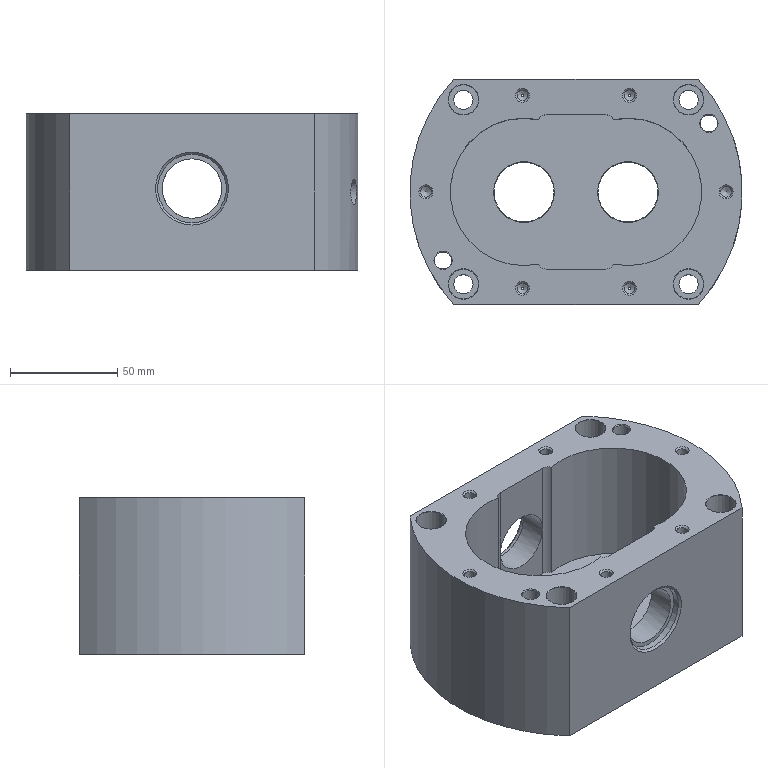NC program | NX | posted with a generic post | part box 155 x 105 x 73.2 mm
Lines 28870 to 29618 of 30727:
(FLOOR_WALL_1_COPY_COPY , TOOL : D12)
N57708 T12 M6
N57710 G54
N57712 G17 G0 G90 X-11.414 Y28.649 B0. C0. S4000 M3
N57714 G43 Z30. H12
N57716 Z-57.2
N57718 G94 G1 Z-60.2 F500.
N57720 G3 X-12.453 Y29.249 R1.2
N57722 G1 X12.453 F1000.
N57724 G3 X18.824 Y27.112 R6.75
N57726 G2 X38.981 Y23.399 R27.65
N57728 G1 X-38.981
N57730 G3 X-45.617 Y17.549 R27.65
N57732 G1 X45.617
N57734 G2 X49.303 Y11.699 R27.65
N57736 G1 X-49.303
N57738 G3 X-51.274 Y5.849 R27.65
N57740 G1 X51.274
N57742 G2 X51.9 Y0. R27.65
N57744 G1 X-51.9
N57746 G3 X-51.274 Y-5.85 R27.65
N57748 G1 X51.274
N57750 G2 X49.302 Y-11.7 R27.65
N57752 G1 X-49.302
N57754 G3 X-45.616 Y-17.55 R27.65
N57756 G1 X45.616
N57758 G2 X38.98 Y-23.4 R27.65
N57760 G1 X-38.98
N57762 G3 X-18.824 Y-27.112 R27.65
N57764 G2 X-12.452 Y-29.25 R6.75
N57766 G1 X12.452
N57768 G3 X12.693 Y-28.074 R1.2
N57770 G1 X12.332 Y-29.838
N57772 G3 X12.901 Y-29.648 R0.6 F500.
N57774 G2 X18.707 Y-27.701 R6.15 F1000.
N57776 G3 X18.707 Y27.701 R-28.25
N57778 G2 X12.729 Y29.85 R6.15
N57780 G1 X-12.729
N57782 G2 X-18.707 Y27.701 R6.15
N57784 G3 X-18.707 Y-27.701 R-28.25
N57786 G2 X-12.729 Y-29.85 R6.15
N57788 G1 X12.729
N57790 G2 X12.901 Y-29.648 R6.15
N57792 G3 X13.142 Y-28.473 R1.2
N57794 G1 X12.371 Y-26.154
N57796 Z-57.2
N57798 G0 Z30.
(ZLEVEL_PROFILE , TOOL : D12)
N57800 X-13.809 Y-22.52 S5000
N57802 Z-13.05
N57804 G1 Z-15.05 F1250.
N57806 X-14.839 Y-24.027
N57808 G3 X-14.93 Y-25.224 R1.2
N57810 G1 X-12.637 Y-30.
N57812 X12.637
N57814 X14.949 Y-25.184
N57816 G3 X14.858 Y-23.987 R1.2
N57818 G1 X13.835 Y-22.489
N57820 Z-13.05
N57822 G0 X-13.832 Y-22.491 Z-28.1
N57824 G1 Z-30.1
N57826 X-14.854 Y-24.026
N57828 G3 X-14.93 Y-25.224 R1.2
N57830 G1 X-14.907 Y-25.269
N57832 X-12.636 Y-30.
N57834 X12.636
N57836 X14.949 Y-25.183
N57838 G3 X14.858 Y-23.987 R1.2
N57840 G1 X13.834 Y-22.489
N57842 Z-28.1
N57844 G0 X-13.809 Y-22.52 Z-43.15
N57846 G1 Z-45.15
N57848 X-14.838 Y-24.027
N57850 G3 X-14.929 Y-25.223 R1.2
N57852 G1 X-12.636 Y-30.
N57854 X12.636
N57856 X14.946 Y-25.189
N57858 G3 X14.854 Y-23.992 R1.2
N57860 G1 X13.83 Y-22.493
N57862 Z-43.15
N57864 G0 X-13.808 Y-22.52 Z-58.2
N57866 G1 Z-60.2
N57868 X-14.838 Y-24.027
N57870 G3 X-14.929 Y-25.223 R1.2
N57872 G1 X-12.635 Y-30.
N57874 X12.635
N57876 X14.945 Y-25.189
N57878 G3 X14.854 Y-23.992 R1.2
N57880 G1 X13.829 Y-22.493
N57882 Z-58.2
N57884 G0 Z30.
N57886 X13.824 Y22.503
N57888 Z-13.05
N57890 G1 Z-15.05
N57892 X14.85 Y24.004
N57894 G3 X14.941 Y25.201 R1.2
N57896 G1 X12.636 Y30.001
N57898 X12.592 Y30.
N57900 X-12.592
N57902 X-12.636 Y30.001
N57904 X-14.93 Y25.224
N57906 G3 X-14.839 Y24.027 R1.2
N57908 G1 X-13.809 Y22.52
N57910 Z-13.05
N57912 G0 X13.823 Y22.503 Z-28.1
N57914 G1 Z-30.1
N57916 X14.85 Y24.004
N57918 G3 X14.941 Y25.201 R1.2
N57920 G1 X12.636 Y30.001
N57922 X12.592 Y30.
N57924 X-12.592
N57926 X-12.636 Y30.001
N57928 X-14.93 Y25.224
N57930 G3 X-14.839 Y24.027 R1.2
N57932 G1 X-13.809 Y22.52
N57934 Z-28.1
N57936 G0 X13.823 Y22.502 Z-43.15
N57938 G1 Z-45.15
N57940 X14.849 Y24.004
N57942 G3 X14.94 Y25.2 R1.2
N57944 G1 X12.636 Y30.
N57946 X-12.636
N57948 X-14.929 Y25.223
N57950 G3 X-14.838 Y24.027 R1.2
N57952 G1 X-13.809 Y22.52
N57954 Z-43.15
N57956 G0 X13.823 Y22.502 Z-58.2
N57958 G1 Z-60.2
N57960 X14.849 Y24.004
N57962 G3 X14.94 Y25.2 R1.2
N57964 G1 X12.635 Y30.
N57966 X-12.635
N57968 X-14.929 Y25.223
N57970 G3 X-14.838 Y24.027 R1.2
N57972 G1 X-13.808 Y22.52
N57974 Z-58.2
N57976 G0 Z30.
N57978 M5
(HOLE_MILLING_COPY_COPY_COPY_COPY , TOOL : D10)
N57980 T10 M6
N57982 G54
N57984 G17 G0 G90 X-52.5 Y43. B0. C0. S3000 M3
N57986 G43 Z30. H10
N57988 Z1.
N57990 G94 G3 X-51.55 Y42.05 R0.95 F2200.
N57992 X-50.6 Y43. R0.95
N57994 X-50.6 Y43. Z0.78 I-1.9 J0.
N57996 X-50.6 Y43. Z0.56 I-1.9 J0.
N57998 X-50.6 Y43. Z0.34 I-1.9 J0.
N58000 X-50.6 Y43. Z0.12 I-1.9 J0.
N58002 X-50.6 Y43. Z-0.1 I-1.9 J0.
N58004 X-50.6 Y43. Z-0.32 I-1.9 J0.
N58006 X-50.6 Y43. Z-0.54 I-1.9 J0.
N58008 X-50.6 Y43. Z-0.76 I-1.9 J0.
N58010 X-50.6 Y43. Z-0.98 I-1.9 J0.
N58012 X-50.6 Y43. Z-1.2 I-1.9 J0.
N58014 X-50.6 Y43. Z-1.42 I-1.9 J0.
N58016 X-50.6 Y43. Z-1.64 I-1.9 J0.
N58018 X-50.6 Y43. Z-1.86 I-1.9 J0.
N58020 X-50.6 Y43. Z-2.08 I-1.9 J0.
N58022 X-50.6 Y43. Z-2.3 I-1.9 J0.
N58024 X-50.6 Y43. Z-2.52 I-1.9 J0.
N58026 X-50.6 Y43. Z-2.74 I-1.9 J0.
N58028 X-50.6 Y43. Z-2.96 I-1.9 J0.
N58030 X-50.6 Y43. Z-3.18 I-1.9 J0.
N58032 X-50.6 Y43. Z-3.4 I-1.9 J0.
N58034 X-50.6 Y43. Z-3.62 I-1.9 J0.
N58036 X-50.6 Y43. Z-3.84 I-1.9 J0.
N58038 X-50.6 Y43. Z-4.06 I-1.9 J0.
N58040 X-50.6 Y43. Z-4.28 I-1.9 J0.
N58042 X-50.6 Y43. Z-4.5 I-1.9 J0.
N58044 X-50.6 Y43. Z-4.72 I-1.9 J0.
N58046 X-50.6 Y43. Z-4.94 I-1.9 J0.
N58048 X-50.6 Y43. Z-5.16 I-1.9 J0.
N58050 X-50.6 Y43. Z-5.38 I-1.9 J0.
N58052 X-50.6 Y43. Z-5.6 I-1.9 J0.
N58054 X-50.6 Y43. Z-5.82 I-1.9 J0.
N58056 X-50.6 Y43. Z-6.04 I-1.9 J0.
N58058 X-50.6 Y43. Z-6.26 I-1.9 J0.
N58060 X-50.6 Y43. Z-6.48 I-1.9 J0.
N58062 X-50.6 Y43. Z-6.7 I-1.9 J0.
N58064 X-50.6 Y43. Z-6.92 I-1.9 J0.
N58066 X-50.6 Y43. Z-7.14 I-1.9 J0.
N58068 X-50.6 Y43. Z-7.36 I-1.9 J0.
N58070 X-50.6 Y43. Z-7.58 I-1.9 J0.
N58072 X-50.6 Y43. Z-7.8 I-1.9 J0.
N58074 X-50.6 Y43. Z-8.02 I-1.9 J0.
N58076 X-50.6 Y43. Z-8.24 I-1.9 J0.
N58078 X-50.6 Y43. Z-8.46 I-1.9 J0.
N58080 X-50.6 Y43. Z-8.68 I-1.9 J0.
N58082 X-50.6 Y43. Z-8.9 I-1.9 J0.
N58084 X-50.6 Y43. Z-9.12 I-1.9 J0.
N58086 X-50.6 Y43. Z-9.34 I-1.9 J0.
N58088 X-50.6 Y43. Z-9.56 I-1.9 J0.
N58090 X-50.6 Y43. Z-9.78 I-1.9 J0.
N58092 X-50.6 Y43. Z-10. I-1.9 J0.
N58094 X-50.6 Y43. Z-10.22 I-1.9 J0.
N58096 X-50.6 Y43. Z-10.44 I-1.9 J0.
N58098 X-50.6 Y43. Z-10.66 I-1.9 J0.
N58100 X-50.6 Y43. Z-10.88 I-1.9 J0.
N58102 X-50.6 Y43. Z-11.1 I-1.9 J0.
N58104 X-50.6 Y43. Z-11.32 I-1.9 J0.
N58106 X-50.6 Y43. Z-11.54 I-1.9 J0.
N58108 X-50.6 Y43. Z-11.76 I-1.9 J0.
N58110 X-50.6 Y43. Z-11.98 I-1.9 J0.
N58112 X-50.6 Y43. Z-12.2 I-1.9 J0.
N58114 X-50.6 Y43. Z-12.42 I-1.9 J0.
N58116 X-50.6 Y43. Z-12.64 I-1.9 J0.
N58118 X-50.6 Y43. Z-12.86 I-1.9 J0.
N58120 X-50.6 Y43. Z-13.08 I-1.9 J0.
N58122 X-50.6 Y43. Z-13.3 I-1.9 J0.
N58124 X-50.6 Y43. Z-13.52 I-1.9 J0.
N58126 X-50.6 Y43. Z-13.74 I-1.9 J0.
N58128 X-50.6 Y43. Z-13.96 I-1.9 J0.
N58130 X-50.6 Y43. Z-14.18 I-1.9 J0.
N58132 X-50.6 Y43. Z-14.4 I-1.9 J0.
N58134 X-50.6 Y43. Z-14.62 I-1.9 J0.
N58136 X-50.6 Y43. Z-14.84 I-1.9 J0.
N58138 X-50.6 Y43. Z-15.06 I-1.9 J0.
N58140 X-50.6 Y43. Z-15.28 I-1.9 J0.
N58142 X-50.6 Y43. Z-15.5 I-1.9 J0.
N58144 X-50.6 Y43. Z-15.72 I-1.9 J0.
N58146 X-50.6 Y43. Z-15.94 I-1.9 J0.
N58148 X-50.6 Y43. Z-16.16 I-1.9 J0.
N58150 X-50.6 Y43. Z-16.38 I-1.9 J0.
N58152 X-50.6 Y43. Z-16.6 I-1.9 J0.
N58154 X-50.6 Y43. Z-16.82 I-1.9 J0.
N58156 X-50.6 Y43. Z-17.04 I-1.9 J0.
N58158 X-50.6 Y43. Z-17.26 I-1.9 J0.
N58160 X-50.6 Y43. Z-17.48 I-1.9 J0.
N58162 X-50.6 Y43. Z-17.7 I-1.9 J0.
N58164 X-50.6 Y43. Z-17.92 I-1.9 J0.
N58166 X-50.6 Y43. Z-18.14 I-1.9 J0.
N58168 X-50.6 Y43. Z-18.36 I-1.9 J0.
N58170 X-50.6 Y43. Z-18.58 I-1.9 J0.
N58172 X-50.6 Y43. Z-18.8 I-1.9 J0.
N58174 X-50.6 Y43. Z-19.02 I-1.9 J0.
N58176 X-50.6 Y43. Z-19.24 I-1.9 J0.
N58178 X-50.6 Y43. Z-19.46 I-1.9 J0.
N58180 X-50.6 Y43. Z-19.68 I-1.9 J0.
N58182 X-50.6 Y43. Z-19.9 I-1.9 J0.
N58184 X-50.6 Y43. Z-20.12 I-1.9 J0.
N58186 X-50.6 Y43. Z-20.34 I-1.9 J0.
N58188 X-50.6 Y43. Z-20.56 I-1.9 J0.
N58190 X-50.6 Y43. Z-20.78 I-1.9 J0.
N58192 X-50.6 Y43. Z-21. I-1.9 J0.
N58194 X-50.6 Y43. Z-21.22 I-1.9 J0.
N58196 X-50.6 Y43. Z-21.44 I-1.9 J0.
N58198 X-50.6 Y43. Z-21.66 I-1.9 J0.
N58200 X-50.6 Y43. Z-21.88 I-1.9 J0.
N58202 X-50.6 Y43. Z-22.1 I-1.9 J0.
N58204 X-50.6 Y43. Z-22.32 I-1.9 J0.
N58206 X-50.6 Y43. Z-22.54 I-1.9 J0.
N58208 X-50.6 Y43. Z-22.76 I-1.9 J0.
N58210 X-50.6 Y43. Z-22.98 I-1.9 J0.
N58212 X-50.6 Y43. Z-23.2 I-1.9 J0.
N58214 X-50.6 Y43. Z-23.42 I-1.9 J0.
N58216 X-50.6 Y43. Z-23.64 I-1.9 J0.
N58218 X-50.6 Y43. Z-23.86 I-1.9 J0.
N58220 X-50.6 Y43. Z-24.08 I-1.9 J0.
N58222 X-50.6 Y43. Z-24.3 I-1.9 J0.
N58224 X-50.6 Y43. Z-24.52 I-1.9 J0.
N58226 X-50.6 Y43. Z-24.74 I-1.9 J0.
N58228 X-50.6 Y43. Z-24.96 I-1.9 J0.
N58230 X-50.6 Y43. Z-25.18 I-1.9 J0.
N58232 X-50.6 Y43. Z-25.4 I-1.9 J0.
N58234 X-50.6 Y43. Z-25.62 I-1.9 J0.
N58236 X-50.6 Y43. Z-25.84 I-1.9 J0.
N58238 X-50.6 Y43. Z-26.06 I-1.9 J0.
N58240 X-50.6 Y43. Z-26.28 I-1.9 J0.
N58242 X-50.6 Y43. Z-26.5 I-1.9 J0.
N58244 X-50.6 Y43. Z-26.72 I-1.9 J0.
N58246 X-50.6 Y43. Z-26.94 I-1.9 J0.
N58248 X-50.6 Y43. Z-27.16 I-1.9 J0.
N58250 X-50.6 Y43. Z-27.38 I-1.9 J0.
N58252 X-50.6 Y43. Z-27.6 I-1.9 J0.
N58254 X-50.6 Y43. Z-27.82 I-1.9 J0.
N58256 X-50.6 Y43. Z-28.04 I-1.9 J0.
N58258 X-50.6 Y43. Z-28.26 I-1.9 J0.
N58260 X-50.6 Y43. Z-28.48 I-1.9 J0.
N58262 X-50.6 Y43. Z-28.7 I-1.9 J0.
N58264 X-50.6 Y43. Z-28.92 I-1.9 J0.
N58266 X-50.6 Y43. Z-29.14 I-1.9 J0.
N58268 X-50.6 Y43. Z-29.36 I-1.9 J0.
N58270 X-50.6 Y43. Z-29.58 I-1.9 J0.
N58272 X-50.6 Y43. Z-29.8 I-1.9 J0.
N58274 X-50.902 Y41.973 Z-30. R-1.9
N58276 X-51.473 Y44.598 R1.9
N58278 X-50.902 Y41.973 R-1.9
N58280 X-51.187 Y43.286 R0.95
N58282 X-52.5 Y43. R0.95
N58284 G0 Z30.
N58286 Y-43.
N58288 Z1.
N58290 G3 X-51.55 Y-43.95 R0.95
N58292 X-50.6 Y-43. R0.95
N58294 X-50.6 Y-43. Z0.78 I-1.9 J0.
N58296 X-50.6 Y-43. Z0.56 I-1.9 J0.
N58298 X-50.6 Y-43. Z0.34 I-1.9 J0.
N58300 X-50.6 Y-43. Z0.12 I-1.9 J0.
N58302 X-50.6 Y-43. Z-0.1 I-1.9 J0.
N58304 X-50.6 Y-43. Z-0.32 I-1.9 J0.
N58306 X-50.6 Y-43. Z-0.54 I-1.9 J0.
N58308 X-50.6 Y-43. Z-0.76 I-1.9 J0.
N58310 X-50.6 Y-43. Z-0.98 I-1.9 J0.
N58312 X-50.6 Y-43. Z-1.2 I-1.9 J0.
N58314 X-50.6 Y-43. Z-1.42 I-1.9 J0.
N58316 X-50.6 Y-43. Z-1.64 I-1.9 J0.
N58318 X-50.6 Y-43. Z-1.86 I-1.9 J0.
N58320 X-50.6 Y-43. Z-2.08 I-1.9 J0.
N58322 X-50.6 Y-43. Z-2.3 I-1.9 J0.
N58324 X-50.6 Y-43. Z-2.52 I-1.9 J0.
N58326 X-50.6 Y-43. Z-2.74 I-1.9 J0.
N58328 X-50.6 Y-43. Z-2.96 I-1.9 J0.
N58330 X-50.6 Y-43. Z-3.18 I-1.9 J0.
N58332 X-50.6 Y-43. Z-3.4 I-1.9 J0.
N58334 X-50.6 Y-43. Z-3.62 I-1.9 J0.
N58336 X-50.6 Y-43. Z-3.84 I-1.9 J0.
N58338 X-50.6 Y-43. Z-4.06 I-1.9 J0.
N58340 X-50.6 Y-43. Z-4.28 I-1.9 J0.
N58342 X-50.6 Y-43. Z-4.5 I-1.9 J0.
N58344 X-50.6 Y-43. Z-4.72 I-1.9 J0.
N58346 X-50.6 Y-43. Z-4.94 I-1.9 J0.
N58348 X-50.6 Y-43. Z-5.16 I-1.9 J0.
N58350 X-50.6 Y-43. Z-5.38 I-1.9 J0.
N58352 X-50.6 Y-43. Z-5.6 I-1.9 J0.
N58354 X-50.6 Y-43. Z-5.82 I-1.9 J0.
N58356 X-50.6 Y-43. Z-6.04 I-1.9 J0.
N58358 X-50.6 Y-43. Z-6.26 I-1.9 J0.
N58360 X-50.6 Y-43. Z-6.48 I-1.9 J0.
N58362 X-50.6 Y-43. Z-6.7 I-1.9 J0.
N58364 X-50.6 Y-43. Z-6.92 I-1.9 J0.
N58366 X-50.6 Y-43. Z-7.14 I-1.9 J0.
N58368 X-50.6 Y-43. Z-7.36 I-1.9 J0.
N58370 X-50.6 Y-43. Z-7.58 I-1.9 J0.
N58372 X-50.6 Y-43. Z-7.8 I-1.9 J0.
N58374 X-50.6 Y-43. Z-8.02 I-1.9 J0.
N58376 X-50.6 Y-43. Z-8.24 I-1.9 J0.
N58378 X-50.6 Y-43. Z-8.46 I-1.9 J0.
N58380 X-50.6 Y-43. Z-8.68 I-1.9 J0.
N58382 X-50.6 Y-43. Z-8.9 I-1.9 J0.
N58384 X-50.6 Y-43. Z-9.12 I-1.9 J0.
N58386 X-50.6 Y-43. Z-9.34 I-1.9 J0.
N58388 X-50.6 Y-43. Z-9.56 I-1.9 J0.
N58390 X-50.6 Y-43. Z-9.78 I-1.9 J0.
N58392 X-50.6 Y-43. Z-10. I-1.9 J0.
N58394 X-50.6 Y-43. Z-10.22 I-1.9 J0.
N58396 X-50.6 Y-43. Z-10.44 I-1.9 J0.
N58398 X-50.6 Y-43. Z-10.66 I-1.9 J0.
N58400 X-50.6 Y-43. Z-10.88 I-1.9 J0.
N58402 X-50.6 Y-43. Z-11.1 I-1.9 J0.
N58404 X-50.6 Y-43. Z-11.32 I-1.9 J0.
N58406 X-50.6 Y-43. Z-11.54 I-1.9 J0.
N58408 X-50.6 Y-43. Z-11.76 I-1.9 J0.
N58410 X-50.6 Y-43. Z-11.98 I-1.9 J0.
N58412 X-50.6 Y-43. Z-12.2 I-1.9 J0.
N58414 X-50.6 Y-43. Z-12.42 I-1.9 J0.
N58416 X-50.6 Y-43. Z-12.64 I-1.9 J0.
N58418 X-50.6 Y-43. Z-12.86 I-1.9 J0.
N58420 X-50.6 Y-43. Z-13.08 I-1.9 J0.
N58422 X-50.6 Y-43. Z-13.3 I-1.9 J0.
N58424 X-50.6 Y-43. Z-13.52 I-1.9 J0.
N58426 X-50.6 Y-43. Z-13.74 I-1.9 J0.
N58428 X-50.6 Y-43. Z-13.96 I-1.9 J0.
N58430 X-50.6 Y-43. Z-14.18 I-1.9 J0.
N58432 X-50.6 Y-43. Z-14.4 I-1.9 J0.
N58434 X-50.6 Y-43. Z-14.62 I-1.9 J0.
N58436 X-50.6 Y-43. Z-14.84 I-1.9 J0.
N58438 X-50.6 Y-43. Z-15.06 I-1.9 J0.
N58440 X-50.6 Y-43. Z-15.28 I-1.9 J0.
N58442 X-50.6 Y-43. Z-15.5 I-1.9 J0.
N58444 X-50.6 Y-43. Z-15.72 I-1.9 J0.
N58446 X-50.6 Y-43. Z-15.94 I-1.9 J0.
N58448 X-50.6 Y-43. Z-16.16 I-1.9 J0.
N58450 X-50.6 Y-43. Z-16.38 I-1.9 J0.
N58452 X-50.6 Y-43. Z-16.6 I-1.9 J0.
N58454 X-50.6 Y-43. Z-16.82 I-1.9 J0.
N58456 X-50.6 Y-43. Z-17.04 I-1.9 J0.
N58458 X-50.6 Y-43. Z-17.26 I-1.9 J0.
N58460 X-50.6 Y-43. Z-17.48 I-1.9 J0.
N58462 X-50.6 Y-43. Z-17.7 I-1.9 J0.
N58464 X-50.6 Y-43. Z-17.92 I-1.9 J0.
N58466 X-50.6 Y-43. Z-18.14 I-1.9 J0.
N58468 X-50.6 Y-43. Z-18.36 I-1.9 J0.
N58470 X-50.6 Y-43. Z-18.58 I-1.9 J0.
N58472 X-50.6 Y-43. Z-18.8 I-1.9 J0.
N58474 X-50.6 Y-43. Z-19.02 I-1.9 J0.
N58476 X-50.6 Y-43. Z-19.24 I-1.9 J0.
N58478 X-50.6 Y-43. Z-19.46 I-1.9 J0.
N58480 X-50.6 Y-43. Z-19.68 I-1.9 J0.
N58482 X-50.6 Y-43. Z-19.9 I-1.9 J0.
N58484 X-50.6 Y-43. Z-20.12 I-1.9 J0.
N58486 X-50.6 Y-43. Z-20.34 I-1.9 J0.
N58488 X-50.6 Y-43. Z-20.56 I-1.9 J0.
N58490 X-50.6 Y-43. Z-20.78 I-1.9 J0.
N58492 X-50.6 Y-43. Z-21. I-1.9 J0.
N58494 X-50.6 Y-43. Z-21.22 I-1.9 J0.
N58496 X-50.6 Y-43. Z-21.44 I-1.9 J0.
N58498 X-50.6 Y-43. Z-21.66 I-1.9 J0.
N58500 X-50.6 Y-43. Z-21.88 I-1.9 J0.
N58502 X-50.6 Y-43. Z-22.1 I-1.9 J0.
N58504 X-50.6 Y-43. Z-22.32 I-1.9 J0.
N58506 X-50.6 Y-43. Z-22.54 I-1.9 J0.
N58508 X-50.6 Y-43. Z-22.76 I-1.9 J0.
N58510 X-50.6 Y-43. Z-22.98 I-1.9 J0.
N58512 X-50.6 Y-43. Z-23.2 I-1.9 J0.
N58514 X-50.6 Y-43. Z-23.42 I-1.9 J0.
N58516 X-50.6 Y-43. Z-23.64 I-1.9 J0.
N58518 X-50.6 Y-43. Z-23.86 I-1.9 J0.
N58520 X-50.6 Y-43. Z-24.08 I-1.9 J0.
N58522 X-50.6 Y-43. Z-24.3 I-1.9 J0.
N58524 X-50.6 Y-43. Z-24.52 I-1.9 J0.
N58526 X-50.6 Y-43. Z-24.74 I-1.9 J0.
N58528 X-50.6 Y-43. Z-24.96 I-1.9 J0.
N58530 X-50.6 Y-43. Z-25.18 I-1.9 J0.
N58532 X-50.6 Y-43. Z-25.4 I-1.9 J0.
N58534 X-50.6 Y-43. Z-25.62 I-1.9 J0.
N58536 X-50.6 Y-43. Z-25.84 I-1.9 J0.
N58538 X-50.6 Y-43. Z-26.06 I-1.9 J0.
N58540 X-50.6 Y-43. Z-26.28 I-1.9 J0.
N58542 X-50.6 Y-43. Z-26.5 I-1.9 J0.
N58544 X-50.6 Y-43. Z-26.72 I-1.9 J0.
N58546 X-50.6 Y-43. Z-26.94 I-1.9 J0.
N58548 X-50.6 Y-43. Z-27.16 I-1.9 J0.
N58550 X-50.6 Y-43. Z-27.38 I-1.9 J0.
N58552 X-50.6 Y-43. Z-27.6 I-1.9 J0.
N58554 X-50.6 Y-43. Z-27.82 I-1.9 J0.
N58556 X-50.6 Y-43. Z-28.04 I-1.9 J0.
N58558 X-50.6 Y-43. Z-28.26 I-1.9 J0.
N58560 X-50.6 Y-43. Z-28.48 I-1.9 J0.
N58562 X-50.6 Y-43. Z-28.7 I-1.9 J0.
N58564 X-50.6 Y-43. Z-28.92 I-1.9 J0.
N58566 X-50.6 Y-43. Z-29.14 I-1.9 J0.
N58568 X-50.6 Y-43. Z-29.36 I-1.9 J0.
N58570 X-50.6 Y-43. Z-29.58 I-1.9 J0.
N58572 X-50.6 Y-43. Z-29.8 I-1.9 J0.
N58574 X-50.902 Y-44.027 Z-30. R-1.9
N58576 X-51.473 Y-41.402 R1.9
N58578 X-50.902 Y-44.027 R-1.9
N58580 X-51.187 Y-42.714 R0.95
N58582 X-52.5 Y-43. R0.95
N58584 G0 Z30.
N58586 X52.5
N58588 Z1.
N58590 G3 X53.45 Y-43.95 R0.95
N58592 X54.4 Y-43. R0.95
N58594 X54.4 Y-43. Z0.78 I-1.9 J0.
N58596 X54.4 Y-43. Z0.56 I-1.9 J0.
N58598 X54.4 Y-43. Z0.34 I-1.9 J0.
N58600 X54.4 Y-43. Z0.12 I-1.9 J0.
N58602 X54.4 Y-43. Z-0.1 I-1.9 J0.
N58604 X54.4 Y-43. Z-0.32 I-1.9 J0.
N58606 X54.4 Y-43. Z-0.54 I-1.9 J0.
N58608 X54.4 Y-43. Z-0.76 I-1.9 J0.
N58610 X54.4 Y-43. Z-0.98 I-1.9 J0.
N58612 X54.4 Y-43. Z-1.2 I-1.9 J0.
N58614 X54.4 Y-43. Z-1.42 I-1.9 J0.
N58616 X54.4 Y-43. Z-1.64 I-1.9 J0.
N58618 X54.4 Y-43. Z-1.86 I-1.9 J0.
N58620 X54.4 Y-43. Z-2.08 I-1.9 J0.
N58622 X54.4 Y-43. Z-2.3 I-1.9 J0.
N58624 X54.4 Y-43. Z-2.52 I-1.9 J0.
N58626 X54.4 Y-43. Z-2.74 I-1.9 J0.
N58628 X54.4 Y-43. Z-2.96 I-1.9 J0.
N58630 X54.4 Y-43. Z-3.18 I-1.9 J0.
N58632 X54.4 Y-43. Z-3.4 I-1.9 J0.
N58634 X54.4 Y-43. Z-3.62 I-1.9 J0.
N58636 X54.4 Y-43. Z-3.84 I-1.9 J0.
N58638 X54.4 Y-43. Z-4.06 I-1.9 J0.
N58640 X54.4 Y-43. Z-4.28 I-1.9 J0.
N58642 X54.4 Y-43. Z-4.5 I-1.9 J0.
N58644 X54.4 Y-43. Z-4.72 I-1.9 J0.
N58646 X54.4 Y-43. Z-4.94 I-1.9 J0.
N58648 X54.4 Y-43. Z-5.16 I-1.9 J0.
N58650 X54.4 Y-43. Z-5.38 I-1.9 J0.
N58652 X54.4 Y-43. Z-5.6 I-1.9 J0.
N58654 X54.4 Y-43. Z-5.82 I-1.9 J0.
N58656 X54.4 Y-43. Z-6.04 I-1.9 J0.
N58658 X54.4 Y-43. Z-6.26 I-1.9 J0.
N58660 X54.4 Y-43. Z-6.48 I-1.9 J0.
N58662 X54.4 Y-43. Z-6.7 I-1.9 J0.
N58664 X54.4 Y-43. Z-6.92 I-1.9 J0.
N58666 X54.4 Y-43. Z-7.14 I-1.9 J0.
N58668 X54.4 Y-43. Z-7.36 I-1.9 J0.
N58670 X54.4 Y-43. Z-7.58 I-1.9 J0.
N58672 X54.4 Y-43. Z-7.8 I-1.9 J0.
N58674 X54.4 Y-43. Z-8.02 I-1.9 J0.
N58676 X54.4 Y-43. Z-8.24 I-1.9 J0.
N58678 X54.4 Y-43. Z-8.46 I-1.9 J0.
N58680 X54.4 Y-43. Z-8.68 I-1.9 J0.
N58682 X54.4 Y-43. Z-8.9 I-1.9 J0.
N58684 X54.4 Y-43. Z-9.12 I-1.9 J0.
N58686 X54.4 Y-43. Z-9.34 I-1.9 J0.
N58688 X54.4 Y-43. Z-9.56 I-1.9 J0.
N58690 X54.4 Y-43. Z-9.78 I-1.9 J0.
N58692 X54.4 Y-43. Z-10. I-1.9 J0.
N58694 X54.4 Y-43. Z-10.22 I-1.9 J0.
N58696 X54.4 Y-43. Z-10.44 I-1.9 J0.
N58698 X54.4 Y-43. Z-10.66 I-1.9 J0.
N58700 X54.4 Y-43. Z-10.88 I-1.9 J0.
N58702 X54.4 Y-43. Z-11.1 I-1.9 J0.
N58704 X54.4 Y-43. Z-11.32 I-1.9 J0.
N58706 X54.4 Y-43. Z-11.54 I-1.9 J0.
N58708 X54.4 Y-43. Z-11.76 I-1.9 J0.
N58710 X54.4 Y-43. Z-11.98 I-1.9 J0.
N58712 X54.4 Y-43. Z-12.2 I-1.9 J0.
N58714 X54.4 Y-43. Z-12.42 I-1.9 J0.
N58716 X54.4 Y-43. Z-12.64 I-1.9 J0.
N58718 X54.4 Y-43. Z-12.86 I-1.9 J0.
N58720 X54.4 Y-43. Z-13.08 I-1.9 J0.
N58722 X54.4 Y-43. Z-13.3 I-1.9 J0.
N58724 X54.4 Y-43. Z-13.52 I-1.9 J0.
N58726 X54.4 Y-43. Z-13.74 I-1.9 J0.
N58728 X54.4 Y-43. Z-13.96 I-1.9 J0.
N58730 X54.4 Y-43. Z-14.18 I-1.9 J0.
N58732 X54.4 Y-43. Z-14.4 I-1.9 J0.
N58734 X54.4 Y-43. Z-14.62 I-1.9 J0.
N58736 X54.4 Y-43. Z-14.84 I-1.9 J0.
N58738 X54.4 Y-43. Z-15.06 I-1.9 J0.
N58740 X54.4 Y-43. Z-15.28 I-1.9 J0.
N58742 X54.4 Y-43. Z-15.5 I-1.9 J0.
N58744 X54.4 Y-43. Z-15.72 I-1.9 J0.
N58746 X54.4 Y-43. Z-15.94 I-1.9 J0.
N58748 X54.4 Y-43. Z-16.16 I-1.9 J0.
N58750 X54.4 Y-43. Z-16.38 I-1.9 J0.
N58752 X54.4 Y-43. Z-16.6 I-1.9 J0.
N58754 X54.4 Y-43. Z-16.82 I-1.9 J0.
N58756 X54.4 Y-43. Z-17.04 I-1.9 J0.
N58758 X54.4 Y-43. Z-17.26 I-1.9 J0.
N58760 X54.4 Y-43. Z-17.48 I-1.9 J0.
N58762 X54.4 Y-43. Z-17.7 I-1.9 J0.
N58764 X54.4 Y-43. Z-17.92 I-1.9 J0.
N58766 X54.4 Y-43. Z-18.14 I-1.9 J0.
N58768 X54.4 Y-43. Z-18.36 I-1.9 J0.
N58770 X54.4 Y-43. Z-18.58 I-1.9 J0.
N58772 X54.4 Y-43. Z-18.8 I-1.9 J0.
N58774 X54.4 Y-43. Z-19.02 I-1.9 J0.
N58776 X54.4 Y-43. Z-19.24 I-1.9 J0.
N58778 X54.4 Y-43. Z-19.46 I-1.9 J0.
N58780 X54.4 Y-43. Z-19.68 I-1.9 J0.
N58782 X54.4 Y-43. Z-19.9 I-1.9 J0.
N58784 X54.4 Y-43. Z-20.12 I-1.9 J0.
N58786 X54.4 Y-43. Z-20.34 I-1.9 J0.
N58788 X54.4 Y-43. Z-20.56 I-1.9 J0.
N58790 X54.4 Y-43. Z-20.78 I-1.9 J0.
N58792 X54.4 Y-43. Z-21. I-1.9 J0.
N58794 X54.4 Y-43. Z-21.22 I-1.9 J0.
N58796 X54.4 Y-43. Z-21.44 I-1.9 J0.
N58798 X54.4 Y-43. Z-21.66 I-1.9 J0.
N58800 X54.4 Y-43. Z-21.88 I-1.9 J0.
N58802 X54.4 Y-43. Z-22.1 I-1.9 J0.
N58804 X54.4 Y-43. Z-22.32 I-1.9 J0.
N58806 X54.4 Y-43. Z-22.54 I-1.9 J0.
N58808 X54.4 Y-43. Z-22.76 I-1.9 J0.
N58810 X54.4 Y-43. Z-22.98 I-1.9 J0.
N58812 X54.4 Y-43. Z-23.2 I-1.9 J0.
N58814 X54.4 Y-43. Z-23.42 I-1.9 J0.
N58816 X54.4 Y-43. Z-23.64 I-1.9 J0.
N58818 X54.4 Y-43. Z-23.86 I-1.9 J0.
N58820 X54.4 Y-43. Z-24.08 I-1.9 J0.
N58822 X54.4 Y-43. Z-24.3 I-1.9 J0.
N58824 X54.4 Y-43. Z-24.52 I-1.9 J0.
N58826 X54.4 Y-43. Z-24.74 I-1.9 J0.
N58828 X54.4 Y-43. Z-24.96 I-1.9 J0.
N58830 X54.4 Y-43. Z-25.18 I-1.9 J0.
N58832 X54.4 Y-43. Z-25.4 I-1.9 J0.
N58834 X54.4 Y-43. Z-25.62 I-1.9 J0.
N58836 X54.4 Y-43. Z-25.84 I-1.9 J0.
N58838 X54.4 Y-43. Z-26.06 I-1.9 J0.
N58840 X54.4 Y-43. Z-26.28 I-1.9 J0.
N58842 X54.4 Y-43. Z-26.5 I-1.9 J0.
N58844 X54.4 Y-43. Z-26.72 I-1.9 J0.
N58846 X54.4 Y-43. Z-26.94 I-1.9 J0.
N58848 X54.4 Y-43. Z-27.16 I-1.9 J0.
N58850 X54.4 Y-43. Z-27.38 I-1.9 J0.
N58852 X54.4 Y-43. Z-27.6 I-1.9 J0.
N58854 X54.4 Y-43. Z-27.82 I-1.9 J0.
N58856 X54.4 Y-43. Z-28.04 I-1.9 J0.
N58858 X54.4 Y-43. Z-28.26 I-1.9 J0.
N58860 X54.4 Y-43. Z-28.48 I-1.9 J0.
N58862 X54.4 Y-43. Z-28.7 I-1.9 J0.
N58864 X54.4 Y-43. Z-28.92 I-1.9 J0.
N58866 X54.4 Y-43. Z-29.14 I-1.9 J0.
N58868 X54.4 Y-43. Z-29.36 I-1.9 J0.
N58870 X54.4 Y-43. Z-29.58 I-1.9 J0.
N58872 X54.4 Y-43. Z-29.8 I-1.9 J0.
N58874 X54.098 Y-44.027 Z-30. R-1.9
N58876 X53.527 Y-41.402 R1.9
N58878 X54.098 Y-44.027 R-1.9
N58880 X53.813 Y-42.714 R0.95
N58882 X52.5 Y-43. R0.95
N58884 G0 Z30.
N58886 Y43.
N58888 Z1.
N58890 G3 X53.45 Y42.05 R0.95
N58892 X54.4 Y43. R0.95
N58894 X54.4 Y43. Z0.78 I-1.9 J0.
N58896 X54.4 Y43. Z0.56 I-1.9 J0.
N58898 X54.4 Y43. Z0.34 I-1.9 J0.
N58900 X54.4 Y43. Z0.12 I-1.9 J0.
N58902 X54.4 Y43. Z-0.1 I-1.9 J0.
N58904 X54.4 Y43. Z-0.32 I-1.9 J0.
N58906 X54.4 Y43. Z-0.54 I-1.9 J0.
N58908 X54.4 Y43. Z-0.76 I-1.9 J0.
N58910 X54.4 Y43. Z-0.98 I-1.9 J0.
N58912 X54.4 Y43. Z-1.2 I-1.9 J0.
N58914 X54.4 Y43. Z-1.42 I-1.9 J0.
N58916 X54.4 Y43. Z-1.64 I-1.9 J0.
N58918 X54.4 Y43. Z-1.86 I-1.9 J0.
N58920 X54.4 Y43. Z-2.08 I-1.9 J0.
N58922 X54.4 Y43. Z-2.3 I-1.9 J0.
N58924 X54.4 Y43. Z-2.52 I-1.9 J0.
N58926 X54.4 Y43. Z-2.74 I-1.9 J0.
N58928 X54.4 Y43. Z-2.96 I-1.9 J0.
N58930 X54.4 Y43. Z-3.18 I-1.9 J0.
N58932 X54.4 Y43. Z-3.4 I-1.9 J0.
N58934 X54.4 Y43. Z-3.62 I-1.9 J0.
N58936 X54.4 Y43. Z-3.84 I-1.9 J0.
N58938 X54.4 Y43. Z-4.06 I-1.9 J0.
N58940 X54.4 Y43. Z-4.28 I-1.9 J0.
N58942 X54.4 Y43. Z-4.5 I-1.9 J0.
N58944 X54.4 Y43. Z-4.72 I-1.9 J0.
N58946 X54.4 Y43. Z-4.94 I-1.9 J0.
N58948 X54.4 Y43. Z-5.16 I-1.9 J0.
N58950 X54.4 Y43. Z-5.38 I-1.9 J0.
N58952 X54.4 Y43. Z-5.6 I-1.9 J0.
N58954 X54.4 Y43. Z-5.82 I-1.9 J0.
N58956 X54.4 Y43. Z-6.04 I-1.9 J0.
N58958 X54.4 Y43. Z-6.26 I-1.9 J0.
N58960 X54.4 Y43. Z-6.48 I-1.9 J0.
N58962 X54.4 Y43. Z-6.7 I-1.9 J0.
N58964 X54.4 Y43. Z-6.92 I-1.9 J0.
N58966 X54.4 Y43. Z-7.14 I-1.9 J0.
N58968 X54.4 Y43. Z-7.36 I-1.9 J0.
N58970 X54.4 Y43. Z-7.58 I-1.9 J0.
N58972 X54.4 Y43. Z-7.8 I-1.9 J0.
N58974 X54.4 Y43. Z-8.02 I-1.9 J0.
N58976 X54.4 Y43. Z-8.24 I-1.9 J0.
N58978 X54.4 Y43. Z-8.46 I-1.9 J0.
N58980 X54.4 Y43. Z-8.68 I-1.9 J0.
N58982 X54.4 Y43. Z-8.9 I-1.9 J0.
N58984 X54.4 Y43. Z-9.12 I-1.9 J0.
N58986 X54.4 Y43. Z-9.34 I-1.9 J0.
N58988 X54.4 Y43. Z-9.56 I-1.9 J0.
N58990 X54.4 Y43. Z-9.78 I-1.9 J0.
N58992 X54.4 Y43. Z-10. I-1.9 J0.
N58994 X54.4 Y43. Z-10.22 I-1.9 J0.
N58996 X54.4 Y43. Z-10.44 I-1.9 J0.
N58998 X54.4 Y43. Z-10.66 I-1.9 J0.
N59000 X54.4 Y43. Z-10.88 I-1.9 J0.
N59002 X54.4 Y43. Z-11.1 I-1.9 J0.
N59004 X54.4 Y43. Z-11.32 I-1.9 J0.
N59006 X54.4 Y43. Z-11.54 I-1.9 J0.
N59008 X54.4 Y43. Z-11.76 I-1.9 J0.
N59010 X54.4 Y43. Z-11.98 I-1.9 J0.
N59012 X54.4 Y43. Z-12.2 I-1.9 J0.
N59014 X54.4 Y43. Z-12.42 I-1.9 J0.
N59016 X54.4 Y43. Z-12.64 I-1.9 J0.
N59018 X54.4 Y43. Z-12.86 I-1.9 J0.
N59020 X54.4 Y43. Z-13.08 I-1.9 J0.
N59022 X54.4 Y43. Z-13.3 I-1.9 J0.
N59024 X54.4 Y43. Z-13.52 I-1.9 J0.
N59026 X54.4 Y43. Z-13.74 I-1.9 J0.
N59028 X54.4 Y43. Z-13.96 I-1.9 J0.
N59030 X54.4 Y43. Z-14.18 I-1.9 J0.
N59032 X54.4 Y43. Z-14.4 I-1.9 J0.
N59034 X54.4 Y43. Z-14.62 I-1.9 J0.
N59036 X54.4 Y43. Z-14.84 I-1.9 J0.
N59038 X54.4 Y43. Z-15.06 I-1.9 J0.
N59040 X54.4 Y43. Z-15.28 I-1.9 J0.
N59042 X54.4 Y43. Z-15.5 I-1.9 J0.
N59044 X54.4 Y43. Z-15.72 I-1.9 J0.
N59046 X54.4 Y43. Z-15.94 I-1.9 J0.
N59048 X54.4 Y43. Z-16.16 I-1.9 J0.
N59050 X54.4 Y43. Z-16.38 I-1.9 J0.
N59052 X54.4 Y43. Z-16.6 I-1.9 J0.
N59054 X54.4 Y43. Z-16.82 I-1.9 J0.
N59056 X54.4 Y43. Z-17.04 I-1.9 J0.
N59058 X54.4 Y43. Z-17.26 I-1.9 J0.
N59060 X54.4 Y43. Z-17.48 I-1.9 J0.
N59062 X54.4 Y43. Z-17.7 I-1.9 J0.
N59064 X54.4 Y43. Z-17.92 I-1.9 J0.
N59066 X54.4 Y43. Z-18.14 I-1.9 J0.
N59068 X54.4 Y43. Z-18.36 I-1.9 J0.
N59070 X54.4 Y43. Z-18.58 I-1.9 J0.
N59072 X54.4 Y43. Z-18.8 I-1.9 J0.
N59074 X54.4 Y43. Z-19.02 I-1.9 J0.
N59076 X54.4 Y43. Z-19.24 I-1.9 J0.
N59078 X54.4 Y43. Z-19.46 I-1.9 J0.
N59080 X54.4 Y43. Z-19.68 I-1.9 J0.
N59082 X54.4 Y43. Z-19.9 I-1.9 J0.
N59084 X54.4 Y43. Z-20.12 I-1.9 J0.
N59086 X54.4 Y43. Z-20.34 I-1.9 J0.
N59088 X54.4 Y43. Z-20.56 I-1.9 J0.
N59090 X54.4 Y43. Z-20.78 I-1.9 J0.
N59092 X54.4 Y43. Z-21. I-1.9 J0.
N59094 X54.4 Y43. Z-21.22 I-1.9 J0.
N59096 X54.4 Y43. Z-21.44 I-1.9 J0.
N59098 X54.4 Y43. Z-21.66 I-1.9 J0.
N59100 X54.4 Y43. Z-21.88 I-1.9 J0.
N59102 X54.4 Y43. Z-22.1 I-1.9 J0.
N59104 X54.4 Y43. Z-22.32 I-1.9 J0.
N59106 X54.4 Y43. Z-22.54 I-1.9 J0.
N59108 X54.4 Y43. Z-22.76 I-1.9 J0.
N59110 X54.4 Y43. Z-22.98 I-1.9 J0.
N59112 X54.4 Y43. Z-23.2 I-1.9 J0.
N59114 X54.4 Y43. Z-23.42 I-1.9 J0.
N59116 X54.4 Y43. Z-23.64 I-1.9 J0.
N59118 X54.4 Y43. Z-23.86 I-1.9 J0.
N59120 X54.4 Y43. Z-24.08 I-1.9 J0.
N59122 X54.4 Y43. Z-24.3 I-1.9 J0.
N59124 X54.4 Y43. Z-24.52 I-1.9 J0.
N59126 X54.4 Y43. Z-24.74 I-1.9 J0.
N59128 X54.4 Y43. Z-24.96 I-1.9 J0.
N59130 X54.4 Y43. Z-25.18 I-1.9 J0.
N59132 X54.4 Y43. Z-25.4 I-1.9 J0.
N59134 X54.4 Y43. Z-25.62 I-1.9 J0.
N59136 X54.4 Y43. Z-25.84 I-1.9 J0.
N59138 X54.4 Y43. Z-26.06 I-1.9 J0.
N59140 X54.4 Y43. Z-26.28 I-1.9 J0.
N59142 X54.4 Y43. Z-26.5 I-1.9 J0.
N59144 X54.4 Y43. Z-26.72 I-1.9 J0.
N59146 X54.4 Y43. Z-26.94 I-1.9 J0.
N59148 X54.4 Y43. Z-27.16 I-1.9 J0.
N59150 X54.4 Y43. Z-27.38 I-1.9 J0.
N59152 X54.4 Y43. Z-27.6 I-1.9 J0.
N59154 X54.4 Y43. Z-27.82 I-1.9 J0.
N59156 X54.4 Y43. Z-28.04 I-1.9 J0.
N59158 X54.4 Y43. Z-28.26 I-1.9 J0.
N59160 X54.4 Y43. Z-28.48 I-1.9 J0.
N59162 X54.4 Y43. Z-28.7 I-1.9 J0.
N59164 X54.4 Y43. Z-28.92 I-1.9 J0.
N59166 X54.4 Y43. Z-29.14 I-1.9 J0.
N59168 X54.4 Y43. Z-29.36 I-1.9 J0.
N59170 X54.4 Y43. Z-29.58 I-1.9 J0.
N59172 X54.4 Y43. Z-29.8 I-1.9 J0.
N59174 X54.098 Y41.973 Z-30. R-1.9
N59176 X53.527 Y44.598 R1.9
N59178 X54.098 Y41.973 R-1.9
N59180 X53.813 Y43.286 R0.95
N59182 X52.5 Y43. R0.95
N59184 G0 Z30.
N59186 M5